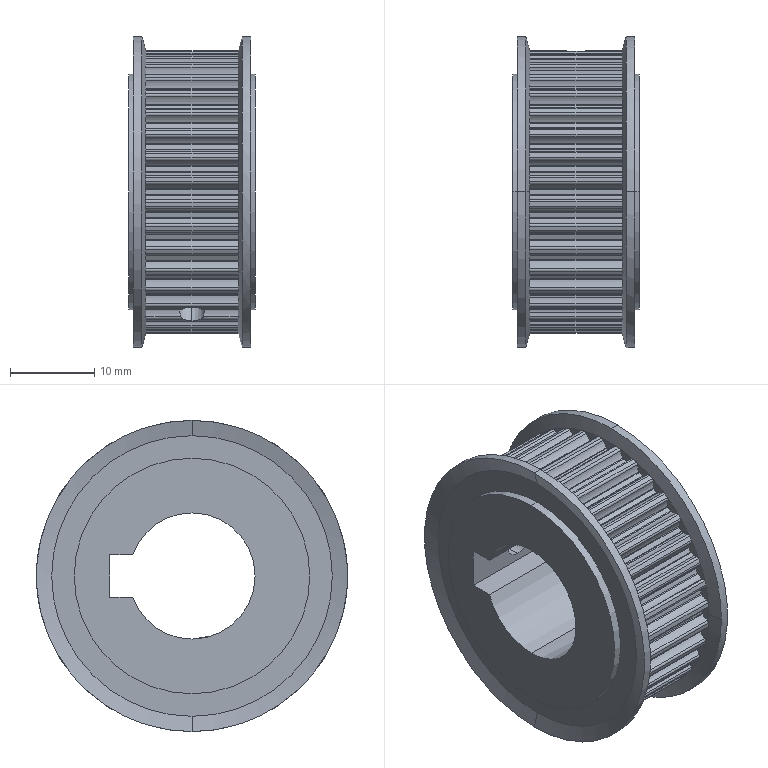Part | STEP file | 11-X_HTPA36S3M100-A-N15-FC37.0_b11 | 1 solid | 438 faces | box 15 x 37 x 37 mm | volume 9550 mm3 | cylinder 351 | plane 79 | cone 8 | commonest cylinder face diameters 0.56 x93 0.3 x86 3.95 x82 31.4 x39 33.62 x36 3.242 x4